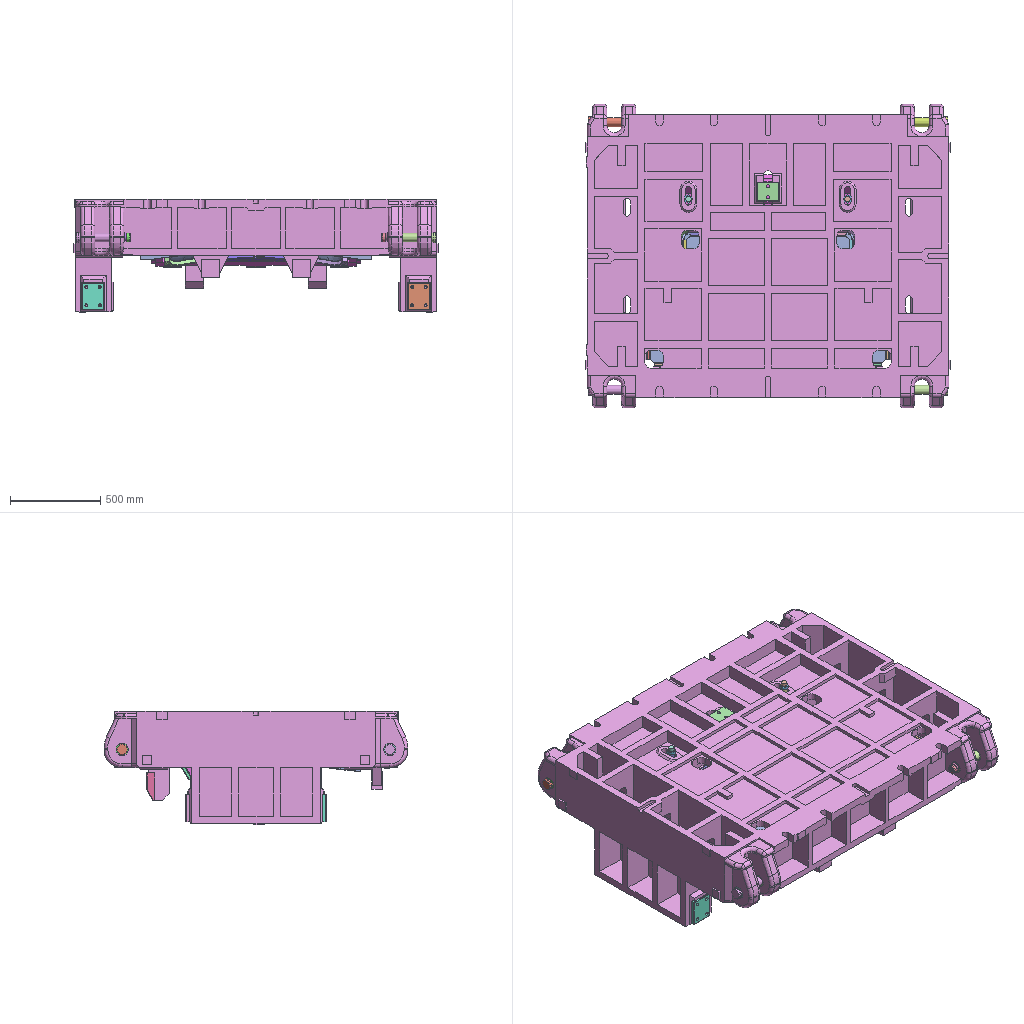Assembly | NX | 119 different items | 119 placed | box 2020 x 1680 x 625 mm
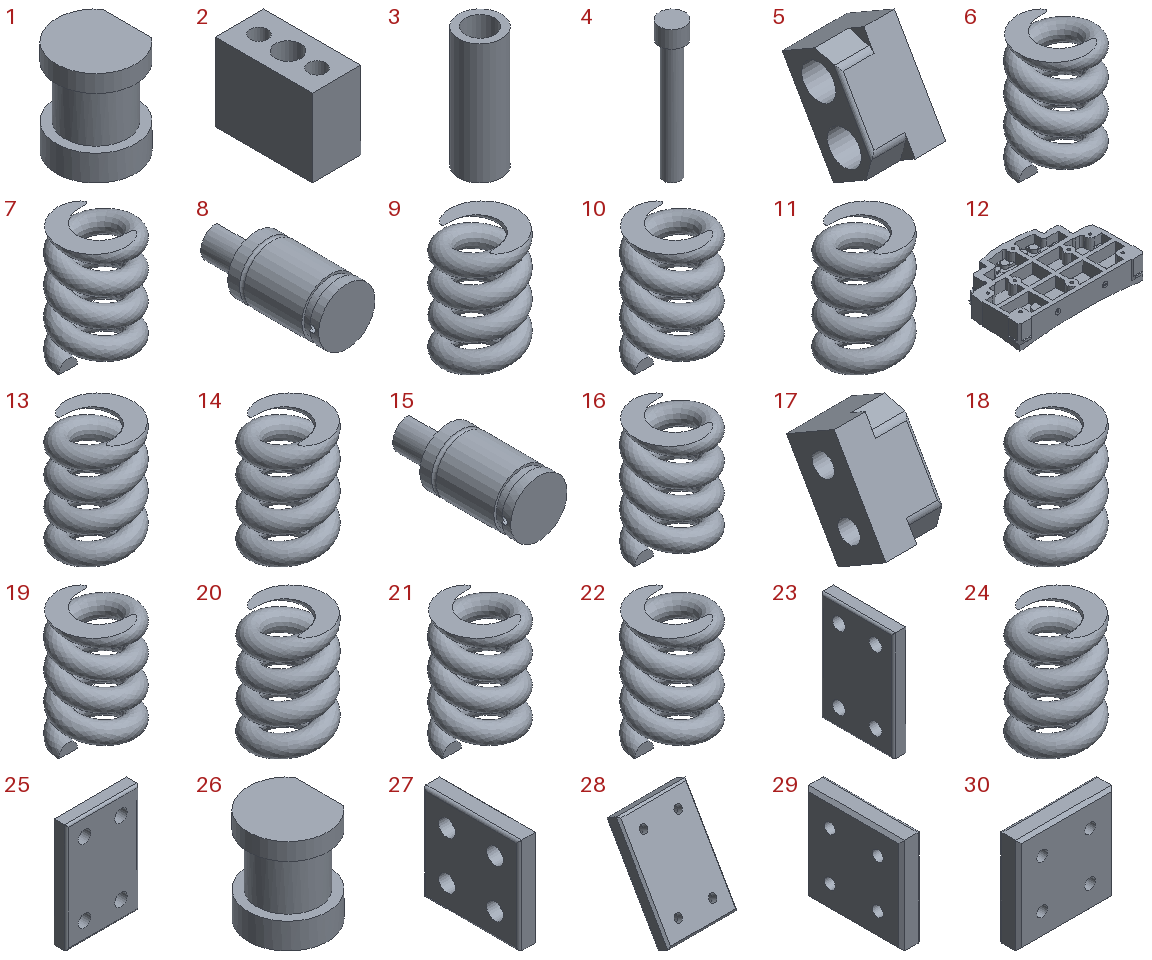Parts list (item | quantity | size | volume | features):
1 | x1 | 46 x 46 x 55 mm | 61296 mm3 | features solid 2
2 | x1 | 50 x 100 x 80 mm | 333398 mm3 | features solid 2
3 | x1 | 32 x 32 x 90 mm | 38790 mm3 | features solid 2
4 | x1 | 30 x 30 x 160 mm | 58119 mm3 | features solid 2
5 | x1 | 38 x 57.713 x 67.962 mm | 55374 mm3 | features MAIN_BODY 2
6 | x1 | 59.9 x 59.795 x 90 mm | 97193 mm3 | features MAIN_BODY 2
7 | x1 | 59.9 x 59.795 x 90 mm | 97193 mm3 | features MAIN_BODY 2
8 | x1 | 50.2 x 116 x 50.2 mm | 169326 mm3 | features MAIN_BODY 2
9 | x1 | 59.9 x 59.795 x 90 mm | 97193 mm3 | features MAIN_BODY 2
10 | x1 | 59.9 x 59.795 x 90 mm | 97193 mm3 | features MAIN_BODY 2
11 | x1 | 59.9 x 59.795 x 90 mm | 97193 mm3 | features MAIN_BODY 2
12 | x1 | 1320 x 831.905 x 257.83 mm | 103011649 mm3 | features solid 2
13 | x1 | 59.9 x 59.795 x 90 mm | 97193 mm3 | features MAIN_BODY 2
14 | x1 | 59.9 x 59.795 x 90 mm | 97193 mm3 | features MAIN_BODY 2
15 | x1 | 50.2 x 116 x 50.2 mm | 169326 mm3 | features MAIN_BODY 2
16 | x1 | 59.9 x 59.795 x 90 mm | 97193 mm3 | features MAIN_BODY 2
17 | x1 | 38 x 57.713 x 67.962 mm | 55374 mm3 | features MAIN_BODY 2
18 | x1 | 59.9 x 59.795 x 90 mm | 97193 mm3 | features MAIN_BODY 2
19 | x1 | 59.9 x 59.795 x 90 mm | 97193 mm3 | features MAIN_BODY 2
20 | x1 | 59.9 x 59.795 x 90 mm | 97193 mm3 | features MAIN_BODY 2
21 | x1 | 59.9 x 59.795 x 90 mm | 97193 mm3 | features MAIN_BODY 2
22 | x1 | 59.9 x 59.795 x 90 mm | 97193 mm3 | features MAIN_BODY 2
23 | x1 | 20 x 100 x 150 mm | 282244 mm3 | features solid 2
24 | x1 | 59.9 x 59.795 x 90 mm | 97193 mm3 | features MAIN_BODY 2
25 | x1 | 100 x 20 x 150 mm | 282244 mm3 | features solid 2
26 | x1 | 46 x 46 x 55 mm | 61296 mm3 | features solid 2
27 | x1 | 20 x 100 x 100 mm | 182887 mm3 | features solid 2
28 | x1 | 100 x 89.722 x 137.306 mm | 282244 mm3 | features solid 2
29 | x1 | 20 x 100 x 100 mm | 182887 mm3 | features solid 2
30 | x1 | 100 x 20 x 100 mm | 182887 mm3 | features solid 2
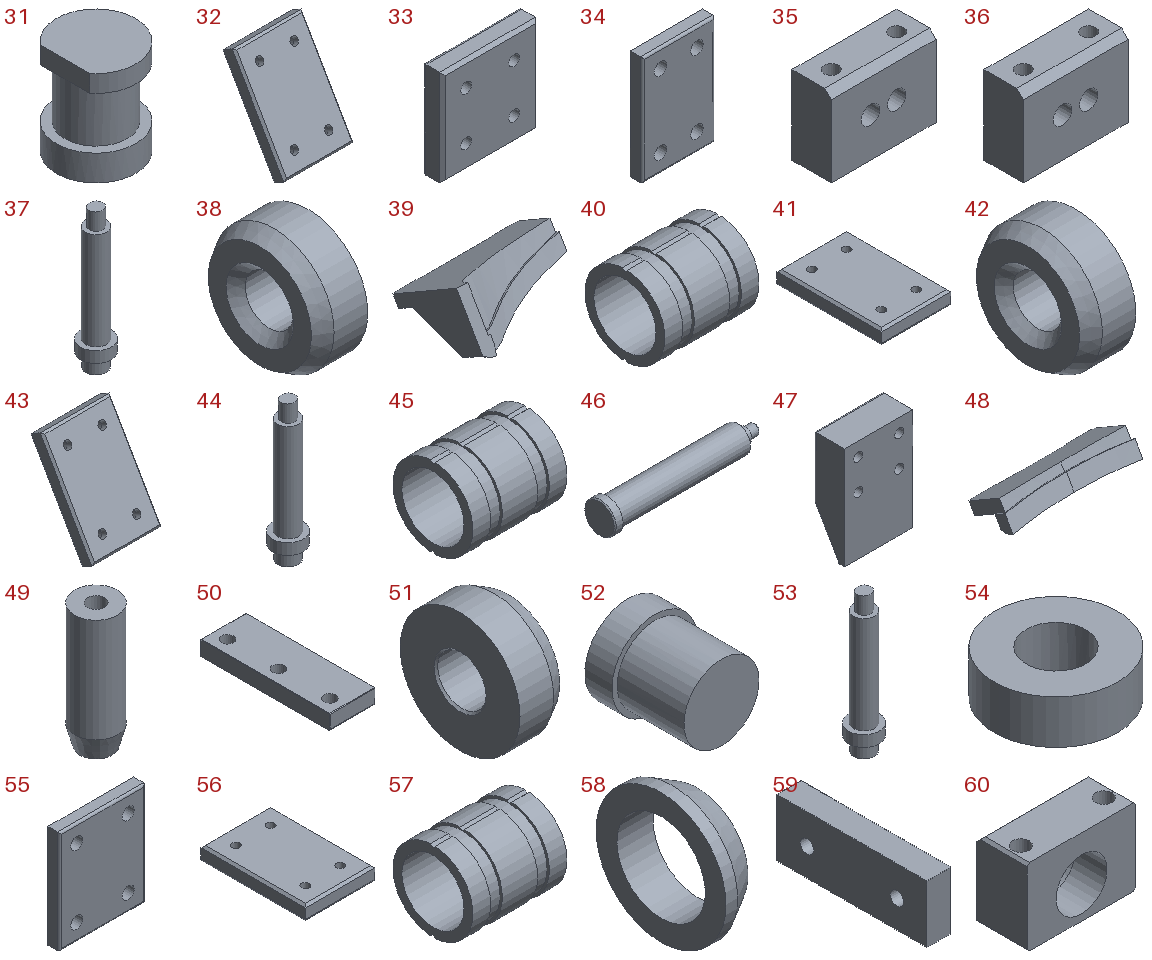31 | x1 | 46 x 46 x 55 mm | 61296 mm3 | features solid 2
32 | x1 | 100 x 89.722 x 137.306 mm | 282244 mm3 | features solid 2
33 | x1 | 100 x 20 x 100 mm | 182887 mm3 | features solid 2
34 | x1 | 100 x 20 x 150 mm | 282244 mm3 | features solid 2
35 | x1 | 80 x 30 x 60 mm | 114333 mm3 | features solid 2
36 | x1 | 80 x 30 x 60 mm | 114333 mm3 | features solid 2
37 | x1 | 36 x 36 x 164 mm | 80942 mm3 | features solid 2
38 | x1 | 20 x 50 x 50 mm | 30708 mm3 | features solid 2
39 | x1 | 336.667 x 251.534 x 153.956 mm | 2324857 mm3 | features solid 2
40 | x1 | 80 x 68 x 67.889 mm | 105275 mm3 | features solid 2
41 | x1 | 100 x 150 x 20 mm | 282244 mm3 | features solid 2
42 | x1 | 20 x 50 x 50 mm | 30708 mm3 | features solid 2
43 | x1 | 100 x 89.722 x 137.306 mm | 282244 mm3 | features solid 2
44 | x1 | 36 x 36 x 164 mm | 80942 mm3 | features solid 2
45 | x1 | 80 x 68 x 67.889 mm | 105275 mm3 | features solid 2
46 | x1 | 300 x 60 x 60 mm | 546127 mm3 | features solid 2
47 | x1 | 100 x 45 x 150 mm | 520948 mm3 | features solid 2
48 | x1 | 336.667 x 123.505 x 74.124 mm | 1242593 mm3 | features solid 2
49 | x1 | 28 x 28 x 80 mm | 39777 mm3 | features solid 2
50 | x1 | 85 x 240 x 28 mm | 538397 mm3 | features solid 2
51 | x1 | 20 x 50 x 50 mm | 30708 mm3 | features solid 2
52 | x1 | 41 x 45 x 41 mm | 49735 mm3 | features solid 2
53 | x1 | 36 x 36 x 164 mm | 80942 mm3 | features solid 2
54 | x1 | 45 x 45 x 16 mm | 19475 mm3 | features solid 2
55 | x1 | 125 x 20 x 150 mm | 356923 mm3 | features solid 2
56 | x1 | 100 x 150 x 20 mm | 282244 mm3 | features solid 2
57 | x1 | 80 x 68 x 67.889 mm | 105275 mm3 | features solid 2
58 | x1 | 14 x 50 x 50 mm | 10965 mm3 | features solid 2
59 | x1 | 20 x 125 x 48 mm | 114744 mm3 | features solid 2
60 | x1 | 85 x 40 x 60 mm | 131435 mm3 | features solid 2
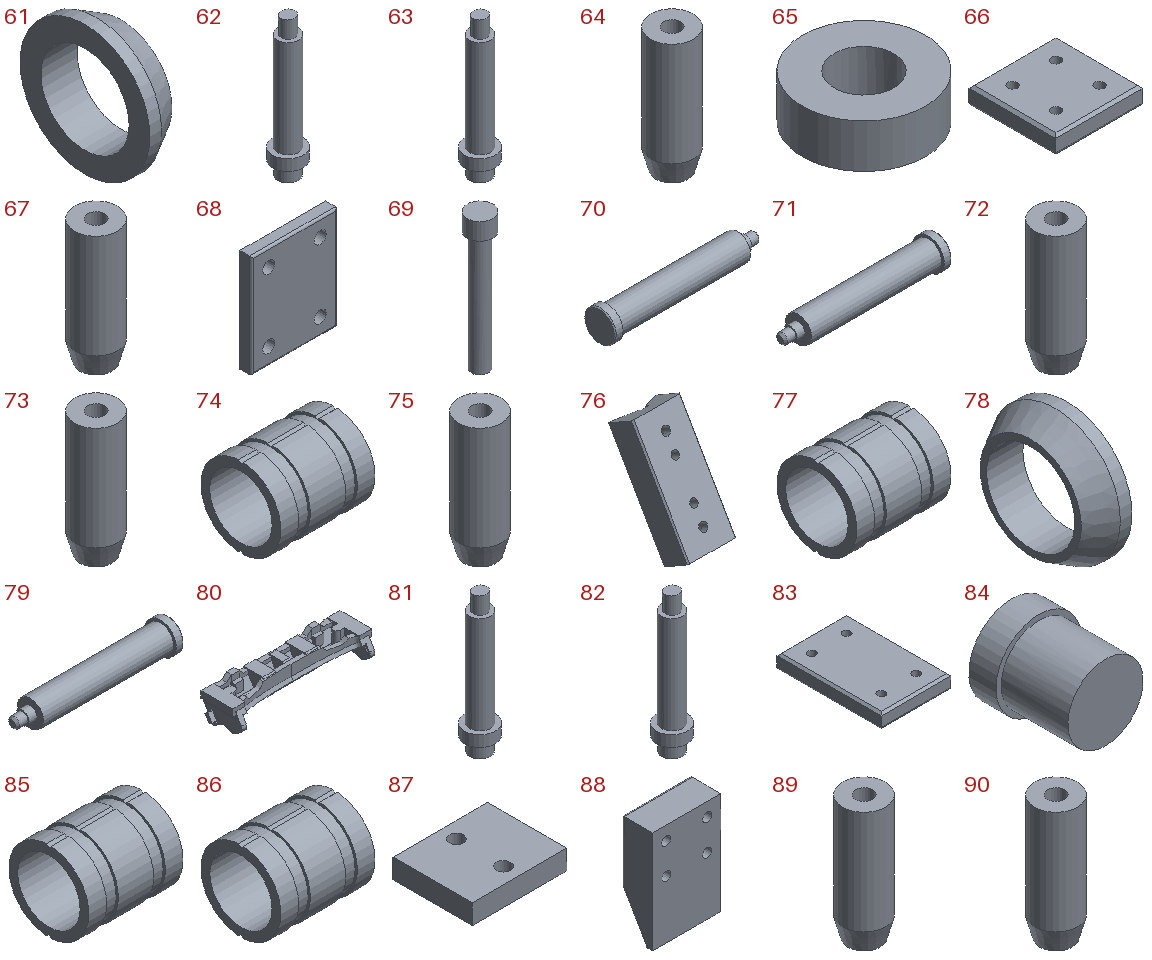61 | x1 | 14 x 50 x 50 mm | 10965 mm3 | features solid 2
62 | x1 | 36 x 36 x 164 mm | 80942 mm3 | features solid 2
63 | x1 | 36 x 36 x 164 mm | 80942 mm3 | features solid 2
64 | x1 | 28 x 28 x 80 mm | 39777 mm3 | features solid 2
65 | x1 | 45 x 45 x 16 mm | 19475 mm3 | features solid 2
66 | x1 | 100 x 100 x 20 mm | 182887 mm3 | features solid 2
67 | x1 | 28 x 28 x 80 mm | 39777 mm3 | features solid 2
68 | x1 | 125 x 20 x 150 mm | 356923 mm3 | features solid 2
69 | x1 | 30 x 30 x 160 mm | 58119 mm3 | features solid 2
70 | x1 | 300 x 60 x 60 mm | 546127 mm3 | features solid 2
71 | x1 | 300 x 60 x 60 mm | 546127 mm3 | features solid 2
72 | x1 | 28 x 28 x 80 mm | 39777 mm3 | features solid 2
73 | x1 | 28 x 28 x 80 mm | 39777 mm3 | features solid 2
74 | x1 | 80 x 68 x 67.889 mm | 105275 mm3 | features solid 2
75 | x1 | 28 x 28 x 80 mm | 39777 mm3 | features solid 2
76 | x1 | 65 x 107.043 x 148.404 mm | 270452 mm3 | features solid 2
77 | x1 | 80 x 68 x 67.889 mm | 105275 mm3 | features solid 2
78 | x1 | 14 x 50 x 50 mm | 10965 mm3 | features solid 2
79 | x1 | 300 x 60 x 60 mm | 546127 mm3 | features solid 2
80 | x1 | 1160 x 335.546 x 254.633 mm | 29497637 mm3 | features solid 2
81 | x1 | 36 x 36 x 164 mm | 80942 mm3 | features solid 2
82 | x1 | 36 x 36 x 164 mm | 80942 mm3 | features solid 2
83 | x1 | 100 x 150 x 20 mm | 282244 mm3 | features solid 2
84 | x1 | 41 x 45 x 41 mm | 49735 mm3 | features solid 2
85 | x1 | 80 x 68 x 67.889 mm | 105275 mm3 | features solid 2
86 | x1 | 80 x 68 x 67.889 mm | 105275 mm3 | features solid 2
87 | x1 | 120 x 100 x 25 mm | 287277 mm3 | features solid 2
88 | x1 | 100 x 45 x 150 mm | 520948 mm3 | features solid 2
89 | x1 | 28 x 28 x 80 mm | 39777 mm3 | features solid 2
90 | x1 | 28 x 28 x 80 mm | 39777 mm3 | features solid 2
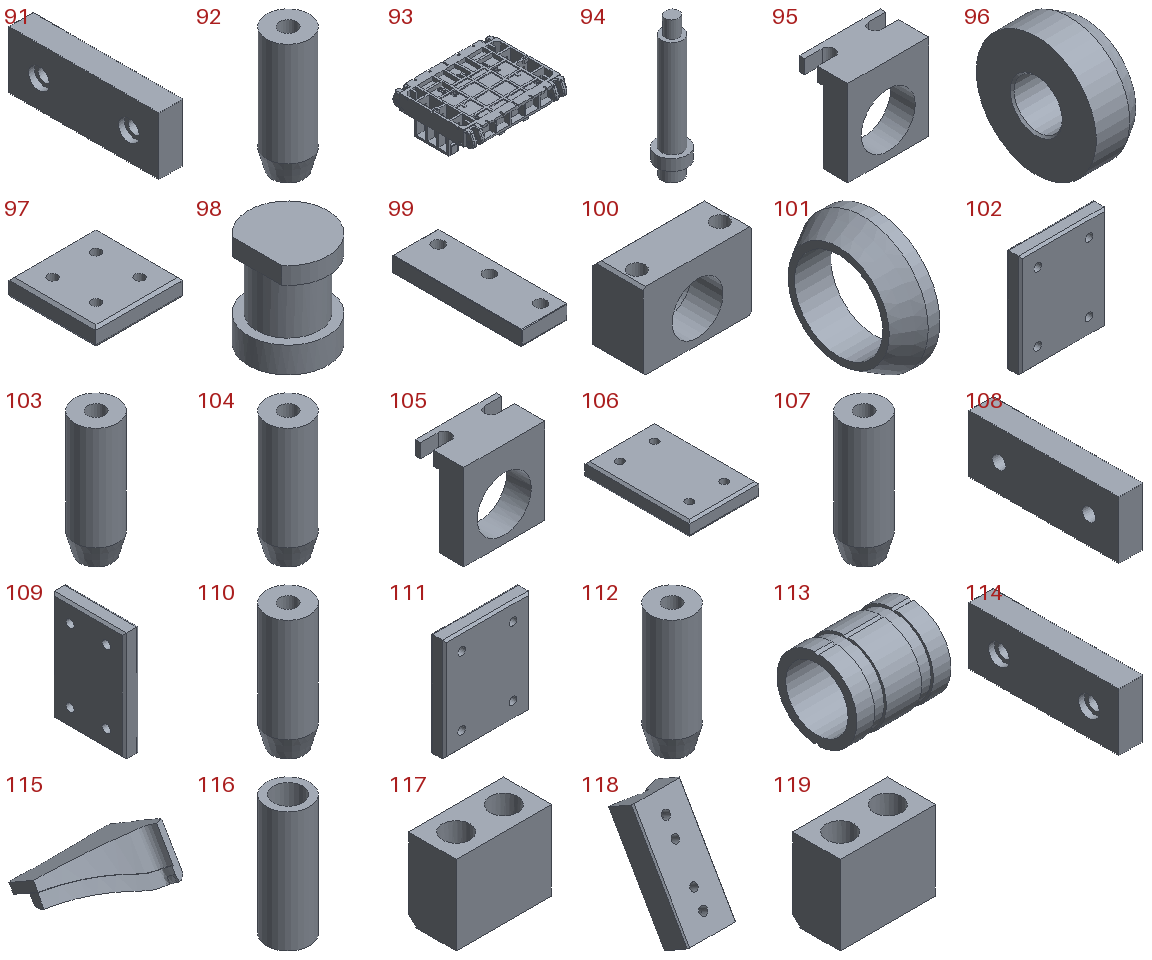91 | x1 | 20 x 125 x 48 mm | 114744 mm3 | features solid 2
92 | x1 | 28 x 28 x 80 mm | 39777 mm3 | features solid 2
93 | x1 | 2020 x 1680 x 625 mm | 373094517 mm3 | features solid 2
94 | x1 | 36 x 36 x 164 mm | 80942 mm3 | features solid 2
95 | x1 | 75 x 45 x 80 mm | 107465 mm3 | features solid 2
96 | x1 | 20 x 50 x 50 mm | 30708 mm3 | features solid 2
97 | x1 | 100 x 100 x 20 mm | 182887 mm3 | features solid 2
98 | x1 | 46 x 46 x 55 mm | 61296 mm3 | features solid 2
99 | x1 | 85 x 240 x 28 mm | 538397 mm3 | features solid 2
100 | x1 | 85 x 40 x 60 mm | 131435 mm3 | features solid 2
101 | x1 | 14 x 50 x 50 mm | 10965 mm3 | features solid 2
102 | x1 | 125 x 20 x 150 mm | 356923 mm3 | features solid 2
103 | x1 | 28 x 28 x 80 mm | 39777 mm3 | features solid 2
104 | x1 | 28 x 28 x 80 mm | 39777 mm3 | features solid 2
105 | x1 | 75 x 45 x 80 mm | 107465 mm3 | features solid 2
106 | x1 | 100 x 150 x 20 mm | 282244 mm3 | features solid 2
107 | x1 | 28 x 28 x 80 mm | 39777 mm3 | features solid 2
108 | x1 | 20 x 125 x 48 mm | 114744 mm3 | features solid 2
109 | x1 | 20 x 100 x 150 mm | 282244 mm3 | features solid 2
110 | x1 | 28 x 28 x 80 mm | 39777 mm3 | features solid 2
111 | x1 | 125 x 20 x 150 mm | 356923 mm3 | features solid 2
112 | x1 | 28 x 28 x 80 mm | 39777 mm3 | features solid 2
113 | x1 | 80 x 68 x 67.889 mm | 105275 mm3 | features solid 2
114 | x1 | 20 x 125 x 48 mm | 114744 mm3 | features solid 2
115 | x1 | 341.667 x 251.534 x 153.956 mm | 2359000 mm3 | features solid 2
116 | x1 | 32 x 32 x 90 mm | 38790 mm3 | features solid 2
117 | x1 | 60 x 30 x 50 mm | 71017 mm3 | features solid 2
118 | x1 | 65 x 107.043 x 148.404 mm | 270452 mm3 | features solid 2
119 | x1 | 60 x 30 x 50 mm | 71017 mm3 | features solid 2